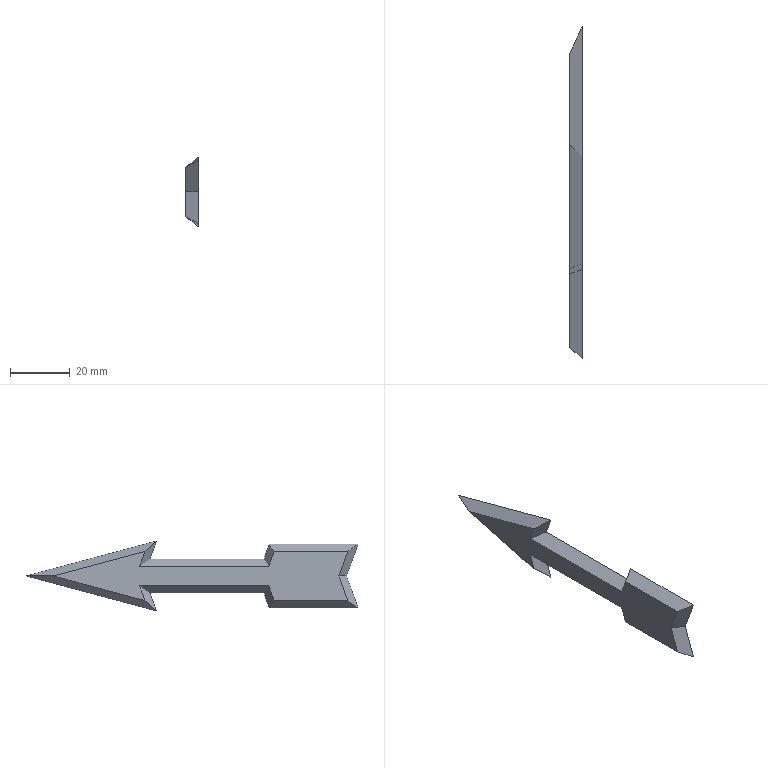Part | NX | features solid 2 | 1 solid | 14 faces | box 4.096 x 110.818 x 23.304 mm | volume 4937 mm3 | plane 14
STEP:
#1=CARTESIAN_POINT('',(-1439.096,-25.454,143.745));
#2=VERTEX_POINT('',#1);
#3=CARTESIAN_POINT('',(-1439.096,-23.665,138.83));
#4=VERTEX_POINT('',#3);
#5=CARTESIAN_POINT('',(-1439.096,-24.559,141.287));
#6=DIRECTION('',(0.,0.342,-0.9397));
#7=VECTOR('',#6,1000.);
#8=LINE('',#5,#7);
#9=EDGE_CURVE('',#2,#4,#8,.T.);
#10=ORIENTED_EDGE('',*,*,#9,.T.);
#11=CARTESIAN_POINT('',(-1439.096,19.49,138.83));
#12=VERTEX_POINT('',#11);
#13=CARTESIAN_POINT('',(-1439.096,-2.087,138.83));
#14=DIRECTION('',(0.,1.,0.));
#15=VECTOR('',#14,1000.);
#16=LINE('',#13,#15);
#17=EDGE_CURVE('',#4,#12,#16,.T.);
#18=ORIENTED_EDGE('',*,*,#17,.T.);
#19=CARTESIAN_POINT('',(-1439.096,17.701,143.745));
#20=VERTEX_POINT('',#19);
#21=CARTESIAN_POINT('',(-1439.096,18.596,141.287));
#22=DIRECTION('',(0.,0.342,-0.9397));
#23=VECTOR('',#22,1000.);
#24=LINE('',#21,#23);
#25=EDGE_CURVE('',#20,#12,#24,.T.);
#26=ORIENTED_EDGE('',*,*,#25,.F.);
#27=CARTESIAN_POINT('',(-1439.096,48.274,135.553));
#28=VERTEX_POINT('',#27);
#29=CARTESIAN_POINT('',(-1439.096,32.988,139.649));
#30=DIRECTION('',(0.,0.9659,-0.2588));
#31=VECTOR('',#30,1000.);
#32=LINE('',#29,#31);
#33=EDGE_CURVE('',#20,#28,#32,.T.);
#34=ORIENTED_EDGE('',*,*,#33,.T.);
#35=CARTESIAN_POINT('',(-1439.096,17.701,127.361));
#36=VERTEX_POINT('',#35);
#37=CARTESIAN_POINT('',(-1439.096,32.988,131.457));
#38=DIRECTION('',(0.,0.9659,0.2588));
#39=VECTOR('',#38,1000.);
#40=LINE('',#37,#39);
#41=EDGE_CURVE('',#36,#28,#40,.T.);
#42=ORIENTED_EDGE('',*,*,#41,.F.);
#43=CARTESIAN_POINT('',(-1439.096,19.49,132.276));
#44=VERTEX_POINT('',#43);
#45=CARTESIAN_POINT('',(-1439.096,18.596,129.819));
#46=DIRECTION('',(0.,0.342,0.9397));
#47=VECTOR('',#46,1000.);
#48=LINE('',#45,#47);
#49=EDGE_CURVE('',#36,#44,#48,.T.);
#50=ORIENTED_EDGE('',*,*,#49,.T.);
#51=CARTESIAN_POINT('',(-1439.096,-23.665,132.276));
#52=VERTEX_POINT('',#51);
#53=CARTESIAN_POINT('',(-1439.096,-2.087,132.276));
#54=DIRECTION('',(0.,1.,0.));
#55=VECTOR('',#54,1000.);
#56=LINE('',#53,#55);
#57=EDGE_CURVE('',#52,#44,#56,.T.);
#58=ORIENTED_EDGE('',*,*,#57,.F.);
#59=CARTESIAN_POINT('',(-1439.096,-25.454,127.361));
#60=VERTEX_POINT('',#59);
#61=CARTESIAN_POINT('',(-1439.096,-24.559,129.819));
#62=DIRECTION('',(0.,0.342,0.9397));
#63=VECTOR('',#62,1000.);
#64=LINE('',#61,#63);
#65=EDGE_CURVE('',#60,#52,#64,.T.);
#66=ORIENTED_EDGE('',*,*,#65,.F.);
#67=CARTESIAN_POINT('',(-1439.096,-50.03,127.361));
#68=VERTEX_POINT('',#67);
#69=CARTESIAN_POINT('',(-1439.096,-37.742,127.361));
#70=DIRECTION('',(0.,1.,0.));
#71=VECTOR('',#70,1000.);
#72=LINE('',#69,#71);
#73=EDGE_CURVE('',#68,#60,#72,.T.);
#74=ORIENTED_EDGE('',*,*,#73,.F.);
#75=CARTESIAN_POINT('',(-1439.096,-47.048,135.553));
#76=VERTEX_POINT('',#75);
#77=CARTESIAN_POINT('',(-1439.096,-48.539,131.457));
#78=DIRECTION('',(0.,0.342,0.9397));
#79=VECTOR('',#78,1000.);
#80=LINE('',#77,#79);
#81=EDGE_CURVE('',#68,#76,#80,.T.);
#82=ORIENTED_EDGE('',*,*,#81,.T.);
#83=CARTESIAN_POINT('',(-1439.096,-50.03,143.745));
#84=VERTEX_POINT('',#83);
#85=CARTESIAN_POINT('',(-1439.096,-48.539,139.649));
#86=DIRECTION('',(0.,0.342,-0.9397));
#87=VECTOR('',#86,1000.);
#88=LINE('',#85,#87);
#89=EDGE_CURVE('',#84,#76,#88,.T.);
#90=ORIENTED_EDGE('',*,*,#89,.F.);
#91=CARTESIAN_POINT('',(-1439.096,-37.742,143.745));
#92=DIRECTION('',(0.,1.,0.));
#93=VECTOR('',#92,1000.);
#94=LINE('',#91,#93);
#95=EDGE_CURVE('',#84,#2,#94,.T.);
#96=ORIENTED_EDGE('',*,*,#95,.T.);
#97=EDGE_LOOP('',(#10,#18,#26,#34,#42,#50,#58,#66,#74,#82,#90,#96));
#98=FACE_BOUND('',#97,.T.);
#99=CARTESIAN_POINT('',(-1439.096,-50.03,135.553));
#100=DIRECTION('',(-1.,0.,0.));
#101=DIRECTION('',(0.,0.,-1.));
#102=AXIS2_PLACEMENT_3D('',#99,#100,#101);
#103=PLANE('',#102);
#104=ADVANCED_FACE('',(#98),#103,.T.);
#105=ORIENTED_EDGE('',*,*,#17,.F.);
#106=CARTESIAN_POINT('',(-1435.,-22.009,141.195));
#107=VERTEX_POINT('',#106);
#108=CARTESIAN_POINT('',(-1437.048,-22.837,140.012));
#109=DIRECTION('',(-0.8174,-0.3304,-0.4719));
#110=VECTOR('',#109,1000.);
#111=LINE('',#108,#110);
#112=EDGE_CURVE('',#107,#4,#111,.T.);
#113=ORIENTED_EDGE('',*,*,#112,.F.);
#114=CARTESIAN_POINT('',(-1435.,16.113,141.195));
#115=VERTEX_POINT('',#114);
#116=CARTESIAN_POINT('',(-1435.,-2.948,141.195));
#117=DIRECTION('',(0.,1.,0.));
#118=VECTOR('',#117,1000.);
#119=LINE('',#116,#118);
#120=EDGE_CURVE('',#107,#115,#119,.T.);
#121=ORIENTED_EDGE('',*,*,#120,.T.);
#122=CARTESIAN_POINT('',(-1437.048,17.802,140.012));
#123=DIRECTION('',(-0.7048,0.5811,-0.4069));
#124=VECTOR('',#123,1000.);
#125=LINE('',#122,#124);
#126=EDGE_CURVE('',#115,#12,#125,.T.);
#127=ORIENTED_EDGE('',*,*,#126,.T.);
#128=EDGE_LOOP('',(#105,#113,#121,#127));
#129=FACE_BOUND('',#128,.T.);
#130=CARTESIAN_POINT('',(-1439.096,19.49,138.83));
#131=DIRECTION('',(0.5,0.,-0.866));
#132=DIRECTION('',(0.866,0.,0.5));
#133=AXIS2_PLACEMENT_3D('',#130,#131,#132);
#134=PLANE('',#133);
#135=ADVANCED_FACE('',(#129),#134,.F.);
#136=ORIENTED_EDGE('',*,*,#25,.T.);
#137=ORIENTED_EDGE('',*,*,#126,.F.);
#138=CARTESIAN_POINT('',(-1435.,13.926,147.205));
#139=VERTEX_POINT('',#138);
#140=CARTESIAN_POINT('',(-1435.,15.019,144.2));
#141=DIRECTION('',(0.,0.342,-0.9397));
#142=VECTOR('',#141,1000.);
#143=LINE('',#140,#142);
#144=EDGE_CURVE('',#139,#115,#143,.T.);
#145=ORIENTED_EDGE('',*,*,#144,.F.);
#146=CARTESIAN_POINT('',(-1437.048,15.814,145.475));
#147=DIRECTION('',(0.6246,-0.5758,0.5276));
#148=VECTOR('',#147,1000.);
#149=LINE('',#146,#148);
#150=EDGE_CURVE('',#20,#139,#149,.T.);
#151=ORIENTED_EDGE('',*,*,#150,.F.);
#152=EDGE_LOOP('',(#136,#137,#145,#151));
#153=FACE_BOUND('',#152,.T.);
#154=CARTESIAN_POINT('',(-1439.096,19.49,138.83));
#155=DIRECTION('',(-0.5,-0.8138,-0.2962));
#156=DIRECTION('',(-0.3387,0.4985,-0.798));
#157=AXIS2_PLACEMENT_3D('',#154,#155,#156);
#158=PLANE('',#157);
#159=ADVANCED_FACE('',(#153),#158,.T.);
#160=ORIENTED_EDGE('',*,*,#33,.F.);
#161=ORIENTED_EDGE('',*,*,#150,.T.);
#162=CARTESIAN_POINT('',(-1435.,57.411,135.553));
#163=VERTEX_POINT('',#162);
#164=CARTESIAN_POINT('',(-1435.,35.668,141.379));
#165=DIRECTION('',(0.,0.9659,-0.2588));
#166=VECTOR('',#165,1000.);
#167=LINE('',#164,#166);
#168=EDGE_CURVE('',#139,#163,#167,.T.);
#169=ORIENTED_EDGE('',*,*,#168,.T.);
#170=CARTESIAN_POINT('',(-1437.048,52.843,135.553));
#171=DIRECTION('',(0.4091,0.9125,0.));
#172=VECTOR('',#171,1000.);
#173=LINE('',#170,#172);
#174=EDGE_CURVE('',#28,#163,#173,.T.);
#175=ORIENTED_EDGE('',*,*,#174,.F.);
#176=EDGE_LOOP('',(#160,#161,#169,#175));
#177=FACE_BOUND('',#176,.T.);
#178=CARTESIAN_POINT('',(-1439.096,48.274,135.553));
#179=DIRECTION('',(0.5,-0.2241,-0.8365));
#180=DIRECTION('',(0.8584,0.,0.5131));
#181=AXIS2_PLACEMENT_3D('',#178,#179,#180);
#182=PLANE('',#181);
#183=ADVANCED_FACE('',(#177),#182,.F.);
#184=ORIENTED_EDGE('',*,*,#41,.T.);
#185=ORIENTED_EDGE('',*,*,#174,.T.);
#186=CARTESIAN_POINT('',(-1435.,13.926,123.901));
#187=VERTEX_POINT('',#186);
#188=CARTESIAN_POINT('',(-1435.,35.668,129.727));
#189=DIRECTION('',(0.,0.9659,0.2588));
#190=VECTOR('',#189,1000.);
#191=LINE('',#188,#190);
#192=EDGE_CURVE('',#187,#163,#191,.T.);
#193=ORIENTED_EDGE('',*,*,#192,.F.);
#194=CARTESIAN_POINT('',(-1437.048,15.814,125.631));
#195=DIRECTION('',(0.6246,-0.5758,-0.5276));
#196=VECTOR('',#195,1000.);
#197=LINE('',#194,#196);
#198=EDGE_CURVE('',#36,#187,#197,.T.);
#199=ORIENTED_EDGE('',*,*,#198,.F.);
#200=EDGE_LOOP('',(#184,#185,#193,#199));
#201=FACE_BOUND('',#200,.T.);
#202=CARTESIAN_POINT('',(-1439.096,48.274,135.553));
#203=DIRECTION('',(-0.5,0.2241,-0.8365));
#204=DIRECTION('',(0.08837,0.9741,0.2082));
#205=AXIS2_PLACEMENT_3D('',#202,#203,#204);
#206=PLANE('',#205);
#207=ADVANCED_FACE('',(#201),#206,.T.);
#208=ORIENTED_EDGE('',*,*,#49,.F.);
#209=ORIENTED_EDGE('',*,*,#198,.T.);
#210=CARTESIAN_POINT('',(-1435.,16.113,129.911));
#211=VERTEX_POINT('',#210);
#212=CARTESIAN_POINT('',(-1435.,15.019,126.906));
#213=DIRECTION('',(0.,0.342,0.9397));
#214=VECTOR('',#213,1000.);
#215=LINE('',#212,#214);
#216=EDGE_CURVE('',#187,#211,#215,.T.);
#217=ORIENTED_EDGE('',*,*,#216,.T.);
#218=CARTESIAN_POINT('',(-1437.048,17.802,131.094));
#219=DIRECTION('',(-0.7048,0.5811,0.4069));
#220=VECTOR('',#219,1000.);
#221=LINE('',#218,#220);
#222=EDGE_CURVE('',#211,#44,#221,.T.);
#223=ORIENTED_EDGE('',*,*,#222,.T.);
#224=EDGE_LOOP('',(#208,#209,#217,#223));
#225=FACE_BOUND('',#224,.T.);
#226=CARTESIAN_POINT('',(-1439.096,19.49,132.276));
#227=DIRECTION('',(0.5,0.8138,-0.2962));
#228=DIRECTION('',(0.7514,-0.5777,-0.3189));
#229=AXIS2_PLACEMENT_3D('',#226,#227,#228);
#230=PLANE('',#229);
#231=ADVANCED_FACE('',(#225),#230,.F.);
#232=ORIENTED_EDGE('',*,*,#57,.T.);
#233=ORIENTED_EDGE('',*,*,#222,.F.);
#234=CARTESIAN_POINT('',(-1435.,-22.009,129.911));
#235=VERTEX_POINT('',#234);
#236=CARTESIAN_POINT('',(-1435.,-2.948,129.911));
#237=DIRECTION('',(0.,1.,0.));
#238=VECTOR('',#237,1000.);
#239=LINE('',#236,#238);
#240=EDGE_CURVE('',#235,#211,#239,.T.);
#241=ORIENTED_EDGE('',*,*,#240,.F.);
#242=CARTESIAN_POINT('',(-1437.048,-22.837,131.094));
#243=DIRECTION('',(0.8174,0.3304,-0.4719));
#244=VECTOR('',#243,1000.);
#245=LINE('',#242,#244);
#246=EDGE_CURVE('',#52,#235,#245,.T.);
#247=ORIENTED_EDGE('',*,*,#246,.F.);
#248=EDGE_LOOP('',(#232,#233,#241,#247));
#249=FACE_BOUND('',#248,.T.);
#250=CARTESIAN_POINT('',(-1439.096,19.49,132.276));
#251=DIRECTION('',(-0.5,0.,-0.866));
#252=DIRECTION('',(0.866,0.,-0.5));
#253=AXIS2_PLACEMENT_3D('',#250,#251,#252);
#254=PLANE('',#253);
#255=ADVANCED_FACE('',(#249),#254,.T.);
#256=ORIENTED_EDGE('',*,*,#65,.T.);
#257=ORIENTED_EDGE('',*,*,#246,.T.);
#258=CARTESIAN_POINT('',(-1435.,-23.798,124.996));
#259=VERTEX_POINT('',#258);
#260=CARTESIAN_POINT('',(-1435.,-22.473,128.636));
#261=DIRECTION('',(0.,0.342,0.9397));
#262=VECTOR('',#261,1000.);
#263=LINE('',#260,#262);
#264=EDGE_CURVE('',#259,#235,#263,.T.);
#265=ORIENTED_EDGE('',*,*,#264,.F.);
#266=CARTESIAN_POINT('',(-1437.048,-24.626,126.179));
#267=DIRECTION('',(-0.8174,-0.3304,0.4719));
#268=VECTOR('',#267,1000.);
#269=LINE('',#266,#268);
#270=EDGE_CURVE('',#259,#60,#269,.T.);
#271=ORIENTED_EDGE('',*,*,#270,.T.);
#272=EDGE_LOOP('',(#256,#257,#265,#271));
#273=FACE_BOUND('',#272,.T.);
#274=CARTESIAN_POINT('',(-1439.096,-23.665,132.276));
#275=DIRECTION('',(-0.5,0.8138,-0.2962));
#276=DIRECTION('',(0.3387,0.4985,0.798));
#277=AXIS2_PLACEMENT_3D('',#274,#275,#276);
#278=PLANE('',#277);
#279=ADVANCED_FACE('',(#273),#278,.T.);
#280=ORIENTED_EDGE('',*,*,#73,.T.);
#281=ORIENTED_EDGE('',*,*,#270,.F.);
#282=CARTESIAN_POINT('',(-1435.,-53.407,124.996));
#283=VERTEX_POINT('',#282);
#284=CARTESIAN_POINT('',(-1435.,-41.478,124.996));
#285=DIRECTION('',(0.,1.,0.));
#286=VECTOR('',#285,1000.);
#287=LINE('',#284,#286);
#288=EDGE_CURVE('',#283,#259,#287,.T.);
#289=ORIENTED_EDGE('',*,*,#288,.F.);
#290=CARTESIAN_POINT('',(-1437.048,-51.718,126.179));
#291=DIRECTION('',(0.7048,-0.5811,-0.4069));
#292=VECTOR('',#291,1000.);
#293=LINE('',#290,#292);
#294=EDGE_CURVE('',#68,#283,#293,.T.);
#295=ORIENTED_EDGE('',*,*,#294,.F.);
#296=EDGE_LOOP('',(#280,#281,#289,#295));
#297=FACE_BOUND('',#296,.T.);
#298=CARTESIAN_POINT('',(-1439.096,-25.454,127.361));
#299=DIRECTION('',(-0.5,0.,-0.866));
#300=DIRECTION('',(0.866,0.,-0.5));
#301=AXIS2_PLACEMENT_3D('',#298,#299,#300);
#302=PLANE('',#301);
#303=ADVANCED_FACE('',(#297),#302,.T.);
#304=ORIENTED_EDGE('',*,*,#81,.F.);
#305=ORIENTED_EDGE('',*,*,#294,.T.);
#306=CARTESIAN_POINT('',(-1435.,-49.565,135.553));
#307=VERTEX_POINT('',#306);
#308=CARTESIAN_POINT('',(-1435.,-51.486,130.275));
#309=DIRECTION('',(0.,0.342,0.9397));
#310=VECTOR('',#309,1000.);
#311=LINE('',#308,#310);
#312=EDGE_CURVE('',#283,#307,#311,.T.);
#313=ORIENTED_EDGE('',*,*,#312,.T.);
#314=CARTESIAN_POINT('',(-1437.048,-48.306,135.553));
#315=DIRECTION('',(-0.852,0.5235,0.));
#316=VECTOR('',#315,1000.);
#317=LINE('',#314,#316);
#318=EDGE_CURVE('',#307,#76,#317,.T.);
#319=ORIENTED_EDGE('',*,*,#318,.T.);
#320=EDGE_LOOP('',(#304,#305,#313,#319));
#321=FACE_BOUND('',#320,.T.);
#322=CARTESIAN_POINT('',(-1439.096,-47.048,135.553));
#323=DIRECTION('',(0.5,0.8138,-0.2962));
#324=DIRECTION('',(0.7514,-0.5777,-0.3189));
#325=AXIS2_PLACEMENT_3D('',#322,#323,#324);
#326=PLANE('',#325);
#327=ADVANCED_FACE('',(#321),#326,.F.);
#328=ORIENTED_EDGE('',*,*,#89,.T.);
#329=ORIENTED_EDGE('',*,*,#318,.F.);
#330=CARTESIAN_POINT('',(-1435.,-53.407,146.11));
#331=VERTEX_POINT('',#330);
#332=CARTESIAN_POINT('',(-1435.,-51.486,140.831));
#333=DIRECTION('',(0.,0.342,-0.9397));
#334=VECTOR('',#333,1000.);
#335=LINE('',#332,#334);
#336=EDGE_CURVE('',#331,#307,#335,.T.);
#337=ORIENTED_EDGE('',*,*,#336,.F.);
#338=CARTESIAN_POINT('',(-1437.048,-51.718,144.927));
#339=DIRECTION('',(0.7048,-0.5811,0.4069));
#340=VECTOR('',#339,1000.);
#341=LINE('',#338,#340);
#342=EDGE_CURVE('',#84,#331,#341,.T.);
#343=ORIENTED_EDGE('',*,*,#342,.F.);
#344=EDGE_LOOP('',(#328,#329,#337,#343));
#345=FACE_BOUND('',#344,.T.);
#346=CARTESIAN_POINT('',(-1439.096,-47.048,135.553));
#347=DIRECTION('',(-0.5,-0.8138,-0.2962));
#348=DIRECTION('',(-0.3387,0.4985,-0.798));
#349=AXIS2_PLACEMENT_3D('',#346,#347,#348);
#350=PLANE('',#349);
#351=ADVANCED_FACE('',(#345),#350,.T.);
#352=ORIENTED_EDGE('',*,*,#95,.F.);
#353=ORIENTED_EDGE('',*,*,#342,.T.);
#354=CARTESIAN_POINT('',(-1435.,-23.798,146.11));
#355=VERTEX_POINT('',#354);
#356=CARTESIAN_POINT('',(-1435.,-38.602,146.11));
#357=DIRECTION('',(0.,1.,0.));
#358=VECTOR('',#357,1000.);
#359=LINE('',#356,#358);
#360=EDGE_CURVE('',#331,#355,#359,.T.);
#361=ORIENTED_EDGE('',*,*,#360,.T.);
#362=CARTESIAN_POINT('',(-1437.048,-24.626,144.927));
#363=DIRECTION('',(-0.8174,-0.3304,-0.4719));
#364=VECTOR('',#363,1000.);
#365=LINE('',#362,#364);
#366=EDGE_CURVE('',#355,#2,#365,.T.);
#367=ORIENTED_EDGE('',*,*,#366,.T.);
#368=EDGE_LOOP('',(#352,#353,#361,#367));
#369=FACE_BOUND('',#368,.T.);
#370=CARTESIAN_POINT('',(-1439.096,-25.454,143.745));
#371=DIRECTION('',(0.5,0.,-0.866));
#372=DIRECTION('',(0.866,0.,0.5));
#373=AXIS2_PLACEMENT_3D('',#370,#371,#372);
#374=PLANE('',#373);
#375=ADVANCED_FACE('',(#369),#374,.F.);
#376=ORIENTED_EDGE('',*,*,#9,.F.);
#377=ORIENTED_EDGE('',*,*,#366,.F.);
#378=CARTESIAN_POINT('',(-1435.,-22.903,143.652));
#379=DIRECTION('',(0.,0.342,-0.9397));
#380=VECTOR('',#379,1000.);
#381=LINE('',#378,#380);
#382=EDGE_CURVE('',#355,#107,#381,.T.);
#383=ORIENTED_EDGE('',*,*,#382,.T.);
#384=ORIENTED_EDGE('',*,*,#112,.T.);
#385=EDGE_LOOP('',(#376,#377,#383,#384));
#386=FACE_BOUND('',#385,.T.);
#387=CARTESIAN_POINT('',(-1439.096,-23.665,138.83));
#388=DIRECTION('',(0.5,-0.8138,-0.2962));
#389=DIRECTION('',(-0.7514,-0.5777,0.3189));
#390=AXIS2_PLACEMENT_3D('',#387,#388,#389);
#391=PLANE('',#390);
#392=ADVANCED_FACE('',(#386),#391,.F.);
#393=ORIENTED_EDGE('',*,*,#120,.F.);
#394=ORIENTED_EDGE('',*,*,#382,.F.);
#395=ORIENTED_EDGE('',*,*,#360,.F.);
#396=ORIENTED_EDGE('',*,*,#336,.T.);
#397=ORIENTED_EDGE('',*,*,#312,.F.);
#398=ORIENTED_EDGE('',*,*,#288,.T.);
#399=ORIENTED_EDGE('',*,*,#264,.T.);
#400=ORIENTED_EDGE('',*,*,#240,.T.);
#401=ORIENTED_EDGE('',*,*,#216,.F.);
#402=ORIENTED_EDGE('',*,*,#192,.T.);
#403=ORIENTED_EDGE('',*,*,#168,.F.);
#404=ORIENTED_EDGE('',*,*,#144,.T.);
#405=EDGE_LOOP('',(#393,#394,#395,#396,#397,#398,#399,#400,#401,#402,#403,#404));
#406=FACE_BOUND('',#405,.T.);
#407=CARTESIAN_POINT('',(-1435.,-29.55,110.977));
#408=DIRECTION('',(-1.,0.,0.));
#409=DIRECTION('',(0.,0.,-1.));
#410=AXIS2_PLACEMENT_3D('',#407,#408,#409);
#411=PLANE('',#410);
#412=ADVANCED_FACE('',(#406),#411,.F.);
#413=CLOSED_SHELL('',(#104,#135,#159,#183,#207,#231,#255,#279,#303,#327,#351,#375,#392,#412));
#414=MANIFOLD_SOLID_BREP('',#413);
#415=(LENGTH_UNIT()NAMED_UNIT(*)SI_UNIT(.MILLI.,.METRE.));
#416=UNCERTAINTY_MEASURE_WITH_UNIT(LENGTH_MEASURE(0.00001),#415,'','');
#417=(NAMED_UNIT(*)PLANE_ANGLE_UNIT()SI_UNIT($,.RADIAN.));
#418=(NAMED_UNIT(*)SI_UNIT($,.STERADIAN.)SOLID_ANGLE_UNIT());
#419=(GEOMETRIC_REPRESENTATION_CONTEXT(3)GLOBAL_UNCERTAINTY_ASSIGNED_CONTEXT((#416))GLOBAL_UNIT_ASSIGNED_CONTEXT((#415,#417,#418))REPRESENTATION_CONTEXT('',''));
#420=ADVANCED_BREP_SHAPE_REPRESENTATION('',(#414),#419);